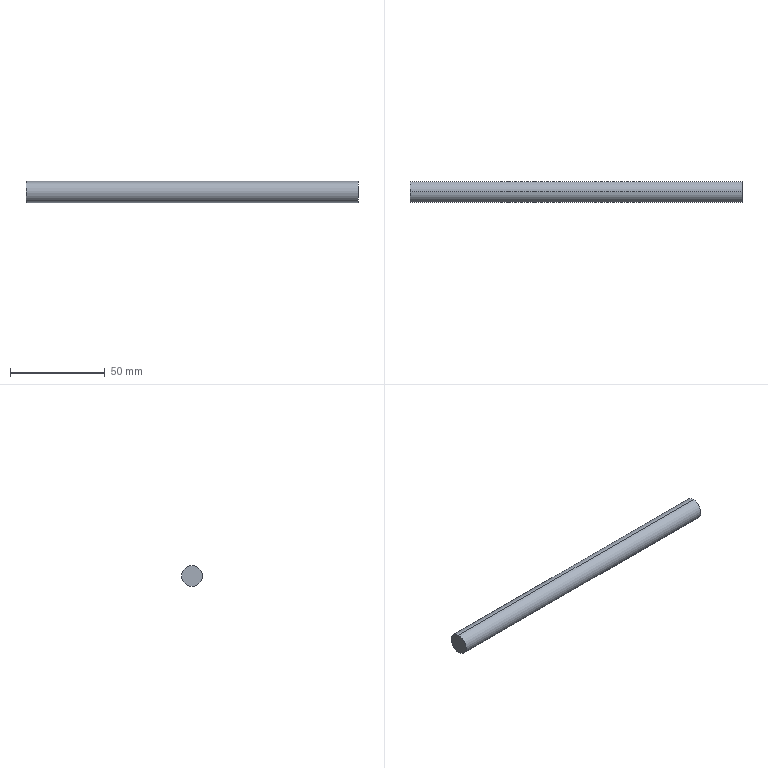Part | STEP file | 4-20.sldasm-Part-388 | 1 solid | 4 faces | box 175 x 11.11 x 11.11 mm | volume 16965 mm3 | cylinder 2 | plane 2 | commonest cylinder face diameters 11.11 x2
STEP:
#1=CARTESIAN_POINT('',(-50.,-60.,198.445));
#2=VERTEX_POINT('',#1);
#3=CARTESIAN_POINT('',(-50.,-60.,209.555));
#4=VERTEX_POINT('',#3);
#5=CARTESIAN_POINT('',(-50.,-60.,204.));
#6=DIRECTION('',(-1.,0.,0.));
#7=DIRECTION('',(0.,0.,1.));
#8=AXIS2_PLACEMENT_3D('',#5,#6,#7);
#9=CIRCLE('',#8,5.555);
#10=EDGE_CURVE('',#2,#4,#9,.T.);
#11=ORIENTED_EDGE('',*,*,#10,.F.);
#12=CARTESIAN_POINT('',(125.,-60.,198.445));
#13=VERTEX_POINT('',#12);
#14=CARTESIAN_POINT('',(50.,-60.,198.445));
#15=DIRECTION('',(1.,0.,0.));
#16=VECTOR('',#15,1000.);
#17=LINE('',#14,#16);
#18=EDGE_CURVE('',#2,#13,#17,.T.);
#19=ORIENTED_EDGE('',*,*,#18,.T.);
#20=CARTESIAN_POINT('',(125.,-60.,209.555));
#21=VERTEX_POINT('',#20);
#22=CARTESIAN_POINT('',(125.,-60.,204.));
#23=DIRECTION('',(1.,0.,0.));
#24=DIRECTION('',(0.,0.,-1.));
#25=AXIS2_PLACEMENT_3D('',#22,#23,#24);
#26=CIRCLE('',#25,5.555);
#27=EDGE_CURVE('',#21,#13,#26,.T.);
#28=ORIENTED_EDGE('',*,*,#27,.F.);
#29=CARTESIAN_POINT('',(50.,-60.,209.555));
#30=DIRECTION('',(1.,0.,0.));
#31=VECTOR('',#30,1000.);
#32=LINE('',#29,#31);
#33=EDGE_CURVE('',#4,#21,#32,.T.);
#34=ORIENTED_EDGE('',*,*,#33,.F.);
#35=EDGE_LOOP('',(#11,#19,#28,#34));
#36=FACE_OUTER_BOUND('',#35,.T.);
#37=CARTESIAN_POINT('',(50.,-60.,204.));
#38=DIRECTION('',(1.,0.,0.));
#39=DIRECTION('',(0.,0.,1.));
#40=AXIS2_PLACEMENT_3D('',#37,#38,#39);
#41=CYLINDRICAL_SURFACE('',#40,5.555);
#42=ADVANCED_FACE('',(#36),#41,.T.);
#43=ORIENTED_EDGE('',*,*,#18,.F.);
#44=CARTESIAN_POINT('',(-50.,-60.,204.));
#45=DIRECTION('',(-1.,0.,0.));
#46=DIRECTION('',(0.,0.,1.));
#47=AXIS2_PLACEMENT_3D('',#44,#45,#46);
#48=CIRCLE('',#47,5.555);
#49=EDGE_CURVE('',#4,#2,#48,.T.);
#50=ORIENTED_EDGE('',*,*,#49,.F.);
#51=ORIENTED_EDGE('',*,*,#33,.T.);
#52=CARTESIAN_POINT('',(125.,-60.,204.));
#53=DIRECTION('',(1.,0.,0.));
#54=DIRECTION('',(0.,0.,-1.));
#55=AXIS2_PLACEMENT_3D('',#52,#53,#54);
#56=CIRCLE('',#55,5.555);
#57=EDGE_CURVE('',#13,#21,#56,.T.);
#58=ORIENTED_EDGE('',*,*,#57,.F.);
#59=EDGE_LOOP('',(#43,#50,#51,#58));
#60=FACE_OUTER_BOUND('',#59,.T.);
#61=CARTESIAN_POINT('',(50.,-60.,204.));
#62=DIRECTION('',(1.,0.,0.));
#63=DIRECTION('',(0.,0.,1.));
#64=AXIS2_PLACEMENT_3D('',#61,#62,#63);
#65=CYLINDRICAL_SURFACE('',#64,5.555);
#66=ADVANCED_FACE('',(#60),#65,.T.);
#67=ORIENTED_EDGE('',*,*,#49,.T.);
#68=ORIENTED_EDGE('',*,*,#10,.T.);
#69=EDGE_LOOP('',(#67,#68));
#70=FACE_OUTER_BOUND('',#69,.T.);
#71=CARTESIAN_POINT('',(-50.,-60.,204.));
#72=DIRECTION('',(-1.,0.,0.));
#73=DIRECTION('',(0.,0.,-1.));
#74=AXIS2_PLACEMENT_3D('',#71,#72,#73);
#75=PLANE('',#74);
#76=ADVANCED_FACE('',(#70),#75,.T.);
#77=ORIENTED_EDGE('',*,*,#27,.T.);
#78=ORIENTED_EDGE('',*,*,#57,.T.);
#79=EDGE_LOOP('',(#77,#78));
#80=FACE_OUTER_BOUND('',#79,.T.);
#81=CARTESIAN_POINT('',(125.,310.,404.));
#82=DIRECTION('',(1.,0.,0.));
#83=DIRECTION('',(0.,0.,-1.));
#84=AXIS2_PLACEMENT_3D('',#81,#82,#83);
#85=PLANE('',#84);
#86=ADVANCED_FACE('',(#80),#85,.T.);
#87=CLOSED_SHELL('',(#42,#66,#76,#86));
#88=MANIFOLD_SOLID_BREP('',#87);
#89=CARTESIAN_POINT('',(0.,0.,0.));
#90=DIRECTION('',(0.,0.,1.));
#91=DIRECTION('',(1.,0.,0.));
#92=AXIS2_PLACEMENT_3D('',#89,#90,#91);
#93=(LENGTH_UNIT()NAMED_UNIT(*)SI_UNIT(.MILLI.,.METRE.));
#94=UNCERTAINTY_MEASURE_WITH_UNIT(LENGTH_MEASURE(0.00001),#93,'','');
#95=(NAMED_UNIT(*)PLANE_ANGLE_UNIT()SI_UNIT($,.RADIAN.));
#96=(NAMED_UNIT(*)SI_UNIT($,.STERADIAN.)SOLID_ANGLE_UNIT());
#97=(GEOMETRIC_REPRESENTATION_CONTEXT(3)GLOBAL_UNCERTAINTY_ASSIGNED_CONTEXT((#94))GLOBAL_UNIT_ASSIGNED_CONTEXT((#93,#95,#96))REPRESENTATION_CONTEXT('',''));
#98=ADVANCED_BREP_SHAPE_REPRESENTATION('',(#88,#92),#97);